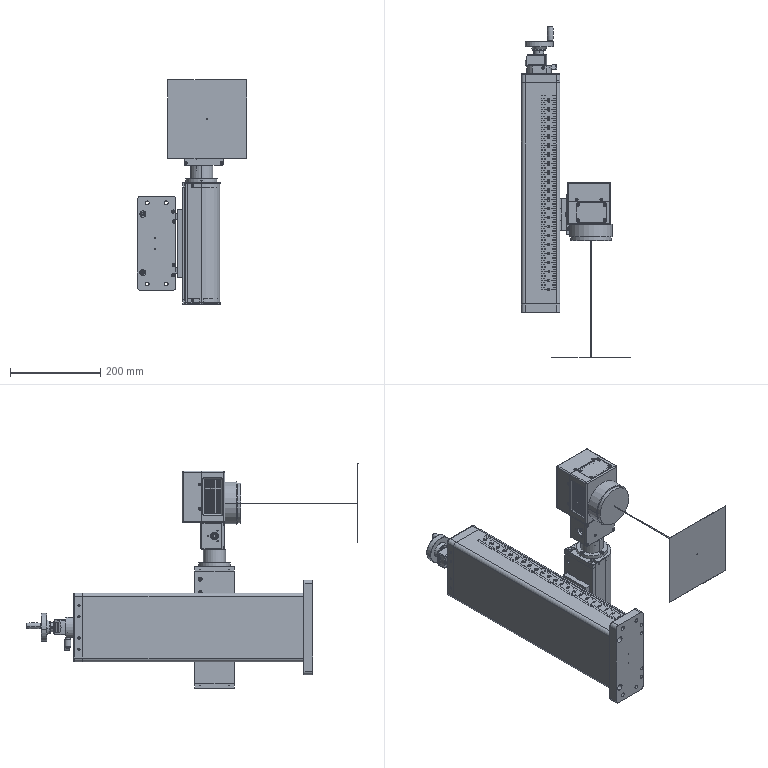Part | SolidWorks | 38 solids | 4736 faces | volume 4821432 mm3 | plane 3137 | cylinder 1077 | cone 296 | spline 205 | sphere 14 | torus 7 | commonest cylinder face diameters 4.5 x92 7.5 x72 2.5 x66 3.3 x62 8 x56 5 x54